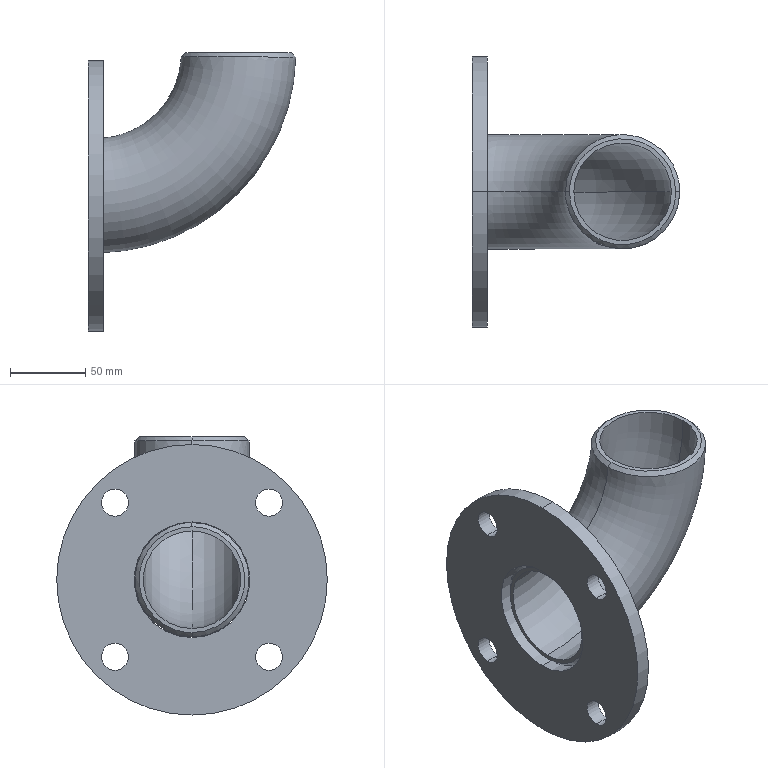Part | SolidWorks | features Chamfer 1, ICE 1, Revolution 1 | 2 solids | 24 faces | box 137.972 x 180 x 185 mm | volume 377579 mm3 | cylinder 12 | spline 4 | torus 4 | plane 4 | commonest cylinder face diameters 18 x8 77 x2 180 x2